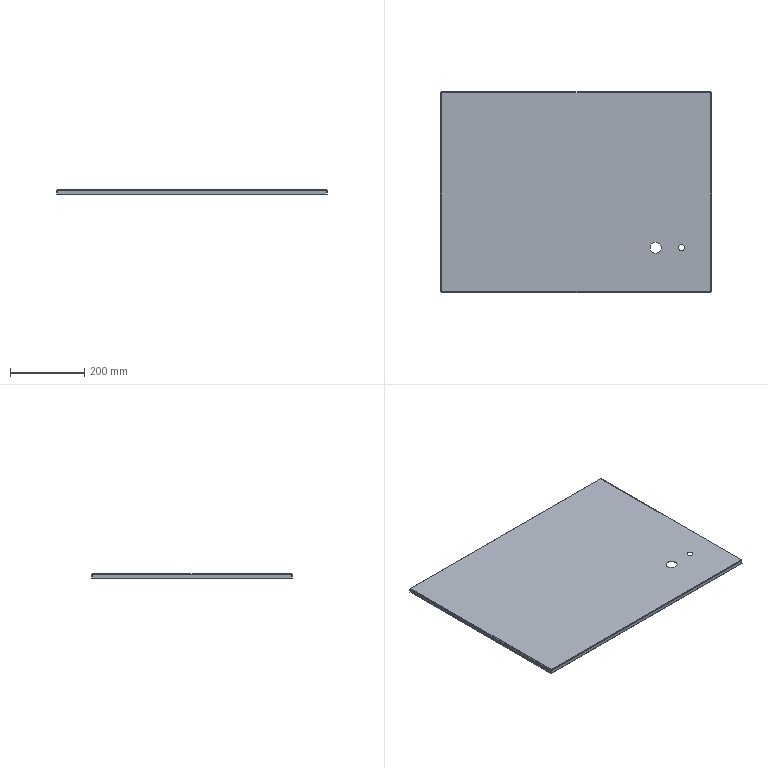Part | SolidWorks | features EdgeFlange 3, FlatPattern 1, ICE 1, SMBaseFlange 1, SMMiteredFlange 1, SheetMetal 1 | 1 solid | 46 faces | box 729.5 x 540 x 11.5 mm | volume 624958 mm3 | plane 34 | cylinder 12 | commonest cylinder face diameters 1.473 x4 4.473 x4 16 x2 30 x2
STEP:
#1=CARTESIAN_POINT('',(276.,-150.,-1.5));
#2=VERTEX_POINT('',#1);
#3=CARTESIAN_POINT('',(292.,-150.,-1.5));
#4=VERTEX_POINT('',#3);
#5=CARTESIAN_POINT('',(284.,-150.,-1.5));
#6=DIRECTION('',(0.,0.,1.));
#7=DIRECTION('',(1.,0.,0.));
#8=AXIS2_PLACEMENT_3D('',#5,#6,#7);
#9=CIRCLE('',#8,8.);
#10=EDGE_CURVE('',#2,#4,#9,.T.);
#11=ORIENTED_EDGE('',*,*,#10,.F.);
#12=CARTESIAN_POINT('',(276.,-150.,0.));
#13=VERTEX_POINT('',#12);
#14=CARTESIAN_POINT('',(276.,-150.,-11.5));
#15=DIRECTION('',(0.,0.,1.));
#16=VECTOR('',#15,1000.);
#17=LINE('',#14,#16);
#18=EDGE_CURVE('',#2,#13,#17,.T.);
#19=ORIENTED_EDGE('',*,*,#18,.T.);
#20=CARTESIAN_POINT('',(292.,-150.,0.));
#21=VERTEX_POINT('',#20);
#22=CARTESIAN_POINT('',(284.,-150.,0.));
#23=DIRECTION('',(0.,0.,1.));
#24=DIRECTION('',(1.,0.,0.));
#25=AXIS2_PLACEMENT_3D('',#22,#23,#24);
#26=CIRCLE('',#25,8.);
#27=EDGE_CURVE('',#13,#21,#26,.T.);
#28=ORIENTED_EDGE('',*,*,#27,.T.);
#29=CARTESIAN_POINT('',(292.,-150.,-11.5));
#30=DIRECTION('',(0.,0.,1.));
#31=VECTOR('',#30,1000.);
#32=LINE('',#29,#31);
#33=EDGE_CURVE('',#4,#21,#32,.T.);
#34=ORIENTED_EDGE('',*,*,#33,.F.);
#35=EDGE_LOOP('',(#11,#19,#28,#34));
#36=FACE_OUTER_BOUND('',#35,.T.);
#37=CARTESIAN_POINT('',(284.,-150.,-11.5));
#38=DIRECTION('',(0.,0.,1.));
#39=DIRECTION('',(1.,0.,0.));
#40=AXIS2_PLACEMENT_3D('',#37,#38,#39);
#41=CYLINDRICAL_SURFACE('',#40,8.);
#42=ADVANCED_FACE('',(#36),#41,.F.);
#43=CARTESIAN_POINT('',(199.,-150.,-1.5));
#44=VERTEX_POINT('',#43);
#45=CARTESIAN_POINT('',(229.,-150.,-1.5));
#46=VERTEX_POINT('',#45);
#47=CARTESIAN_POINT('',(214.,-150.,-1.5));
#48=DIRECTION('',(0.,0.,1.));
#49=DIRECTION('',(1.,0.,0.));
#50=AXIS2_PLACEMENT_3D('',#47,#48,#49);
#51=CIRCLE('',#50,15.);
#52=EDGE_CURVE('',#44,#46,#51,.T.);
#53=ORIENTED_EDGE('',*,*,#52,.F.);
#54=CARTESIAN_POINT('',(199.,-150.,0.));
#55=VERTEX_POINT('',#54);
#56=CARTESIAN_POINT('',(199.,-150.,-11.5));
#57=DIRECTION('',(0.,0.,1.));
#58=VECTOR('',#57,1000.);
#59=LINE('',#56,#58);
#60=EDGE_CURVE('',#44,#55,#59,.T.);
#61=ORIENTED_EDGE('',*,*,#60,.T.);
#62=CARTESIAN_POINT('',(229.,-150.,0.));
#63=VERTEX_POINT('',#62);
#64=CARTESIAN_POINT('',(214.,-150.,0.));
#65=DIRECTION('',(0.,0.,1.));
#66=DIRECTION('',(1.,0.,0.));
#67=AXIS2_PLACEMENT_3D('',#64,#65,#66);
#68=CIRCLE('',#67,15.);
#69=EDGE_CURVE('',#55,#63,#68,.T.);
#70=ORIENTED_EDGE('',*,*,#69,.T.);
#71=CARTESIAN_POINT('',(229.,-150.,-11.5));
#72=DIRECTION('',(0.,0.,1.));
#73=VECTOR('',#72,1000.);
#74=LINE('',#71,#73);
#75=EDGE_CURVE('',#46,#63,#74,.T.);
#76=ORIENTED_EDGE('',*,*,#75,.F.);
#77=EDGE_LOOP('',(#53,#61,#70,#76));
#78=FACE_OUTER_BOUND('',#77,.T.);
#79=CARTESIAN_POINT('',(214.,-150.,-11.5));
#80=DIRECTION('',(0.,0.,1.));
#81=DIRECTION('',(1.,0.,0.));
#82=AXIS2_PLACEMENT_3D('',#79,#80,#81);
#83=CYLINDRICAL_SURFACE('',#82,15.);
#84=ADVANCED_FACE('',(#78),#83,.F.);
#85=CARTESIAN_POINT('',(361.763,268.5,0.));
#86=VERTEX_POINT('',#85);
#87=CARTESIAN_POINT('',(361.763,268.5,-0.1248));
#88=VERTEX_POINT('',#87);
#89=CARTESIAN_POINT('',(361.763,268.5,0.));
#90=DIRECTION('',(0.,0.,-1.));
#91=VECTOR('',#90,1000.);
#92=LINE('',#89,#91);
#93=EDGE_CURVE('',#86,#88,#92,.T.);
#94=ORIENTED_EDGE('',*,*,#93,.T.);
#95=CARTESIAN_POINT('',(361.763,267.763,0.));
#96=VERTEX_POINT('',#95);
#97=CARTESIAN_POINT('',(361.763,267.763,-2.237));
#98=DIRECTION('',(1.,0.,0.));
#99=DIRECTION('',(0.,0.,-1.));
#100=AXIS2_PLACEMENT_3D('',#97,#98,#99);
#101=CIRCLE('',#100,2.237);
#102=EDGE_CURVE('',#88,#96,#101,.T.);
#103=ORIENTED_EDGE('',*,*,#102,.T.);
#104=CARTESIAN_POINT('',(361.763,-2953.5,0.));
#105=DIRECTION('',(0.,1.,0.));
#106=VECTOR('',#105,1000.);
#107=LINE('',#104,#106);
#108=EDGE_CURVE('',#96,#86,#107,.T.);
#109=ORIENTED_EDGE('',*,*,#108,.T.);
#110=EDGE_LOOP('',(#94,#103,#109));
#111=FACE_OUTER_BOUND('',#110,.T.);
#112=CARTESIAN_POINT('',(361.763,268.5,-1.5));
#113=DIRECTION('',(-1.,0.,0.));
#114=DIRECTION('',(0.,0.,1.));
#115=AXIS2_PLACEMENT_3D('',#112,#113,#114);
#116=PLANE('',#115);
#117=ADVANCED_FACE('',(#111),#116,.T.);
#118=CARTESIAN_POINT('',(-363.263,268.5,0.));
#119=VERTEX_POINT('',#118);
#120=CARTESIAN_POINT('',(-363.263,267.763,0.));
#121=VERTEX_POINT('',#120);
#122=CARTESIAN_POINT('',(-363.263,268.5,0.));
#123=DIRECTION('',(0.,-1.,0.));
#124=VECTOR('',#123,1000.);
#125=LINE('',#122,#124);
#126=EDGE_CURVE('',#119,#121,#125,.T.);
#127=ORIENTED_EDGE('',*,*,#126,.T.);
#128=CARTESIAN_POINT('',(-363.263,268.5,-0.1248));
#129=VERTEX_POINT('',#128);
#130=CARTESIAN_POINT('',(-363.263,267.763,-2.237));
#131=DIRECTION('',(-1.,0.,0.));
#132=DIRECTION('',(0.,0.,-1.));
#133=AXIS2_PLACEMENT_3D('',#130,#131,#132);
#134=CIRCLE('',#133,2.237);
#135=EDGE_CURVE('',#121,#129,#134,.T.);
#136=ORIENTED_EDGE('',*,*,#135,.T.);
#137=CARTESIAN_POINT('',(-363.263,268.5,-1.5));
#138=DIRECTION('',(0.,0.,1.));
#139=VECTOR('',#138,1000.);
#140=LINE('',#137,#139);
#141=EDGE_CURVE('',#129,#119,#140,.T.);
#142=ORIENTED_EDGE('',*,*,#141,.T.);
#143=EDGE_LOOP('',(#127,#136,#142));
#144=FACE_OUTER_BOUND('',#143,.T.);
#145=CARTESIAN_POINT('',(-363.263,267.763,-1.5));
#146=DIRECTION('',(1.,0.,0.));
#147=DIRECTION('',(0.,1.,0.));
#148=AXIS2_PLACEMENT_3D('',#145,#146,#147);
#149=PLANE('',#148);
#150=ADVANCED_FACE('',(#144),#149,.T.);
#151=CARTESIAN_POINT('',(284.,-150.,-1.5));
#152=DIRECTION('',(0.,0.,1.));
#153=DIRECTION('',(1.,0.,0.));
#154=AXIS2_PLACEMENT_3D('',#151,#152,#153);
#155=CIRCLE('',#154,8.);
#156=EDGE_CURVE('',#4,#2,#155,.T.);
#157=ORIENTED_EDGE('',*,*,#156,.T.);
#158=ORIENTED_EDGE('',*,*,#10,.T.);
#159=EDGE_LOOP('',(#157,#158));
#160=FACE_BOUND('',#159,.T.);
#161=CARTESIAN_POINT('',(214.,-150.,-1.5));
#162=DIRECTION('',(0.,0.,1.));
#163=DIRECTION('',(1.,0.,0.));
#164=AXIS2_PLACEMENT_3D('',#161,#162,#163);
#165=CIRCLE('',#164,15.);
#166=EDGE_CURVE('',#46,#44,#165,.T.);
#167=ORIENTED_EDGE('',*,*,#166,.T.);
#168=ORIENTED_EDGE('',*,*,#52,.T.);
#169=EDGE_LOOP('',(#167,#168));
#170=FACE_BOUND('',#169,.T.);
#171=CARTESIAN_POINT('',(361.763,267.763,-1.5));
#172=VERTEX_POINT('',#171);
#173=CARTESIAN_POINT('',(-363.263,267.763,-1.5));
#174=VERTEX_POINT('',#173);
#175=CARTESIAN_POINT('',(361.763,267.763,-1.5));
#176=DIRECTION('',(-1.,0.,0.));
#177=VECTOR('',#176,1000.);
#178=LINE('',#175,#177);
#179=EDGE_CURVE('',#172,#174,#178,.T.);
#180=ORIENTED_EDGE('',*,*,#179,.F.);
#181=CARTESIAN_POINT('',(361.763,-267.763,-1.5));
#182=VERTEX_POINT('',#181);
#183=CARTESIAN_POINT('',(361.763,-2953.5,-1.5));
#184=DIRECTION('',(0.,1.,0.));
#185=VECTOR('',#184,1000.);
#186=LINE('',#183,#185);
#187=EDGE_CURVE('',#182,#172,#186,.T.);
#188=ORIENTED_EDGE('',*,*,#187,.F.);
#189=CARTESIAN_POINT('',(-363.263,-267.763,-1.5));
#190=VERTEX_POINT('',#189);
#191=CARTESIAN_POINT('',(-364.,-267.763,-1.5));
#192=DIRECTION('',(1.,0.,0.));
#193=VECTOR('',#192,1000.);
#194=LINE('',#191,#193);
#195=EDGE_CURVE('',#190,#182,#194,.T.);
#196=ORIENTED_EDGE('',*,*,#195,.F.);
#197=CARTESIAN_POINT('',(-363.263,268.5,-1.5));
#198=DIRECTION('',(0.,-1.,0.));
#199=VECTOR('',#198,1000.);
#200=LINE('',#197,#199);
#201=EDGE_CURVE('',#174,#190,#200,.T.);
#202=ORIENTED_EDGE('',*,*,#201,.F.);
#203=EDGE_LOOP('',(#180,#188,#196,#202));
#204=FACE_OUTER_BOUND('',#203,.T.);
#205=CARTESIAN_POINT('',(0.,0.,-1.5));
#206=DIRECTION('',(0.,0.,1.));
#207=DIRECTION('',(1.,0.,0.));
#208=AXIS2_PLACEMENT_3D('',#205,#206,#207);
#209=PLANE('',#208);
#210=ADVANCED_FACE('',(#160,#170,#204),#209,.F.);
#211=CARTESIAN_POINT('',(284.,-150.,0.));
#212=DIRECTION('',(0.,0.,1.));
#213=DIRECTION('',(1.,0.,0.));
#214=AXIS2_PLACEMENT_3D('',#211,#212,#213);
#215=CIRCLE('',#214,8.);
#216=EDGE_CURVE('',#21,#13,#215,.T.);
#217=ORIENTED_EDGE('',*,*,#216,.F.);
#218=ORIENTED_EDGE('',*,*,#27,.F.);
#219=EDGE_LOOP('',(#217,#218));
#220=FACE_BOUND('',#219,.T.);
#221=CARTESIAN_POINT('',(214.,-150.,0.));
#222=DIRECTION('',(0.,0.,1.));
#223=DIRECTION('',(1.,0.,0.));
#224=AXIS2_PLACEMENT_3D('',#221,#222,#223);
#225=CIRCLE('',#224,15.);
#226=EDGE_CURVE('',#63,#55,#225,.T.);
#227=ORIENTED_EDGE('',*,*,#226,.F.);
#228=ORIENTED_EDGE('',*,*,#69,.F.);
#229=EDGE_LOOP('',(#227,#228));
#230=FACE_BOUND('',#229,.T.);
#231=CARTESIAN_POINT('',(361.763,-267.763,0.));
#232=VERTEX_POINT('',#231);
#233=CARTESIAN_POINT('',(361.763,-2953.5,0.));
#234=DIRECTION('',(0.,1.,0.));
#235=VECTOR('',#234,1000.);
#236=LINE('',#233,#235);
#237=EDGE_CURVE('',#232,#96,#236,.T.);
#238=ORIENTED_EDGE('',*,*,#237,.T.);
#239=CARTESIAN_POINT('',(361.763,267.763,0.));
#240=DIRECTION('',(-1.,0.,0.));
#241=VECTOR('',#240,1000.);
#242=LINE('',#239,#241);
#243=EDGE_CURVE('',#96,#121,#242,.T.);
#244=ORIENTED_EDGE('',*,*,#243,.T.);
#245=CARTESIAN_POINT('',(-363.263,-267.763,0.));
#246=VERTEX_POINT('',#245);
#247=CARTESIAN_POINT('',(-363.263,268.5,0.));
#248=DIRECTION('',(0.,-1.,0.));
#249=VECTOR('',#248,1000.);
#250=LINE('',#247,#249);
#251=EDGE_CURVE('',#121,#246,#250,.T.);
#252=ORIENTED_EDGE('',*,*,#251,.T.);
#253=CARTESIAN_POINT('',(-364.,-267.763,0.));
#254=DIRECTION('',(1.,0.,0.));
#255=VECTOR('',#254,1000.);
#256=LINE('',#253,#255);
#257=EDGE_CURVE('',#246,#232,#256,.T.);
#258=ORIENTED_EDGE('',*,*,#257,.T.);
#259=EDGE_LOOP('',(#238,#244,#252,#258));
#260=FACE_OUTER_BOUND('',#259,.T.);
#261=CARTESIAN_POINT('',(0.,0.,0.));
#262=DIRECTION('',(0.,0.,1.));
#263=DIRECTION('',(1.,0.,0.));
#264=AXIS2_PLACEMENT_3D('',#261,#262,#263);
#265=PLANE('',#264);
#266=ADVANCED_FACE('',(#220,#230,#260),#265,.T.);
#267=CARTESIAN_POINT('',(-364.,-267.763,0.));
#268=VERTEX_POINT('',#267);
#269=CARTESIAN_POINT('',(-364.,-267.763,0.));
#270=DIRECTION('',(1.,0.,0.));
#271=VECTOR('',#270,1000.);
#272=LINE('',#269,#271);
#273=EDGE_CURVE('',#268,#246,#272,.T.);
#274=ORIENTED_EDGE('',*,*,#273,.T.);
#275=CARTESIAN_POINT('',(-364.,-267.763,-0.1248));
#276=VERTEX_POINT('',#275);
#277=CARTESIAN_POINT('',(-363.263,-267.763,-2.237));
#278=DIRECTION('',(0.,-1.,0.));
#279=DIRECTION('',(0.,0.,1.));
#280=AXIS2_PLACEMENT_3D('',#277,#278,#279);
#281=CIRCLE('',#280,2.237);
#282=EDGE_CURVE('',#246,#276,#281,.T.);
#283=ORIENTED_EDGE('',*,*,#282,.T.);
#284=CARTESIAN_POINT('',(-364.,-267.763,-1.5));
#285=DIRECTION('',(0.,0.,1.));
#286=VECTOR('',#285,1000.);
#287=LINE('',#284,#286);
#288=EDGE_CURVE('',#276,#268,#287,.T.);
#289=ORIENTED_EDGE('',*,*,#288,.T.);
#290=EDGE_LOOP('',(#274,#283,#289));
#291=FACE_OUTER_BOUND('',#290,.T.);
#292=CARTESIAN_POINT('',(-363.263,-267.763,-1.5));
#293=DIRECTION('',(0.,1.,0.));
#294=DIRECTION('',(-1.,0.,0.));
#295=AXIS2_PLACEMENT_3D('',#292,#293,#294);
#296=PLANE('',#295);
#297=ADVANCED_FACE('',(#291),#296,.T.);
#298=CARTESIAN_POINT('',(361.763,-268.5,0.));
#299=VERTEX_POINT('',#298);
#300=CARTESIAN_POINT('',(361.763,-2953.5,0.));
#301=DIRECTION('',(0.,1.,0.));
#302=VECTOR('',#301,1000.);
#303=LINE('',#300,#302);
#304=EDGE_CURVE('',#299,#232,#303,.T.);
#305=ORIENTED_EDGE('',*,*,#304,.T.);
#306=CARTESIAN_POINT('',(361.763,-268.5,-0.1248));
#307=VERTEX_POINT('',#306);
#308=CARTESIAN_POINT('',(361.763,-267.763,-2.237));
#309=DIRECTION('',(1.,0.,0.));
#310=DIRECTION('',(0.,0.,1.));
#311=AXIS2_PLACEMENT_3D('',#308,#309,#310);
#312=CIRCLE('',#311,2.237);
#313=EDGE_CURVE('',#232,#307,#312,.T.);
#314=ORIENTED_EDGE('',*,*,#313,.T.);
#315=CARTESIAN_POINT('',(361.763,-268.5,0.));
#316=DIRECTION('',(0.,0.,-1.));
#317=VECTOR('',#316,1000.);
#318=LINE('',#315,#317);
#319=EDGE_CURVE('',#299,#307,#318,.T.);
#320=ORIENTED_EDGE('',*,*,#319,.F.);
#321=EDGE_LOOP('',(#305,#314,#320));
#322=FACE_OUTER_BOUND('',#321,.T.);
#323=CARTESIAN_POINT('',(361.763,-267.763,-1.5));
#324=DIRECTION('',(-1.,0.,0.));
#325=DIRECTION('',(0.,-1.,0.));
#326=AXIS2_PLACEMENT_3D('',#323,#324,#325);
#327=PLANE('',#326);
#328=ADVANCED_FACE('',(#322),#327,.T.);
#329=CARTESIAN_POINT('',(364.,268.5,-11.5));
#330=VERTEX_POINT('',#329);
#331=CARTESIAN_POINT('',(362.5,268.5,-11.5));
#332=VERTEX_POINT('',#331);
#333=CARTESIAN_POINT('',(364.,268.5,-11.5));
#334=DIRECTION('',(-1.,0.,0.));
#335=VECTOR('',#334,1000.);
#336=LINE('',#333,#335);
#337=EDGE_CURVE('',#330,#332,#336,.T.);
#338=ORIENTED_EDGE('',*,*,#337,.F.);
#339=CARTESIAN_POINT('',(364.,-268.5,-11.5));
#340=VERTEX_POINT('',#339);
#341=CARTESIAN_POINT('',(364.,-268.5,-11.5));
#342=DIRECTION('',(0.,1.,0.));
#343=VECTOR('',#342,1000.);
#344=LINE('',#341,#343);
#345=EDGE_CURVE('',#340,#330,#344,.T.);
#346=ORIENTED_EDGE('',*,*,#345,.F.);
#347=CARTESIAN_POINT('',(362.5,-268.5,-11.5));
#348=VERTEX_POINT('',#347);
#349=CARTESIAN_POINT('',(364.,-268.5,-11.5));
#350=DIRECTION('',(-1.,0.,0.));
#351=VECTOR('',#350,1000.);
#352=LINE('',#349,#351);
#353=EDGE_CURVE('',#340,#348,#352,.T.);
#354=ORIENTED_EDGE('',*,*,#353,.T.);
#355=CARTESIAN_POINT('',(362.5,-268.5,-11.5));
#356=DIRECTION('',(0.,1.,0.));
#357=VECTOR('',#356,1000.);
#358=LINE('',#355,#357);
#359=EDGE_CURVE('',#348,#332,#358,.T.);
#360=ORIENTED_EDGE('',*,*,#359,.T.);
#361=EDGE_LOOP('',(#338,#346,#354,#360));
#362=FACE_OUTER_BOUND('',#361,.T.);
#363=CARTESIAN_POINT('',(364.,-268.5,-11.5));
#364=DIRECTION('',(0.,0.,1.));
#365=DIRECTION('',(0.,1.,0.));
#366=AXIS2_PLACEMENT_3D('',#363,#364,#365);
#367=PLANE('',#366);
#368=ADVANCED_FACE('',(#362),#367,.F.);
#369=ORIENTED_EDGE('',*,*,#353,.F.);
#370=CARTESIAN_POINT('',(364.,-268.5,-2.237));
#371=VERTEX_POINT('',#370);
#372=CARTESIAN_POINT('',(364.,-268.5,-11.5));
#373=DIRECTION('',(0.,0.,1.));
#374=VECTOR('',#373,1000.);
#375=LINE('',#372,#374);
#376=EDGE_CURVE('',#340,#371,#375,.T.);
#377=ORIENTED_EDGE('',*,*,#376,.T.);
#378=CARTESIAN_POINT('',(362.5,-268.5,-2.237));
#379=VERTEX_POINT('',#378);
#380=CARTESIAN_POINT('',(364.,-268.5,-2.237));
#381=DIRECTION('',(-1.,0.,0.));
#382=VECTOR('',#381,1000.);
#383=LINE('',#380,#382);
#384=EDGE_CURVE('',#371,#379,#383,.T.);
#385=ORIENTED_EDGE('',*,*,#384,.T.);
#386=CARTESIAN_POINT('',(362.5,-268.5,-11.5));
#387=DIRECTION('',(0.,0.,1.));
#388=VECTOR('',#387,1000.);
#389=LINE('',#386,#388);
#390=EDGE_CURVE('',#348,#379,#389,.T.);
#391=ORIENTED_EDGE('',*,*,#390,.F.);
#392=EDGE_LOOP('',(#369,#377,#385,#391));
#393=FACE_OUTER_BOUND('',#392,.T.);
#394=CARTESIAN_POINT('',(364.,-268.5,-11.5));
#395=DIRECTION('',(0.,-1.,0.));
#396=DIRECTION('',(0.,0.,1.));
#397=AXIS2_PLACEMENT_3D('',#394,#395,#396);
#398=PLANE('',#397);
#399=ADVANCED_FACE('',(#393),#398,.T.);
#400=CARTESIAN_POINT('',(364.,268.5,-2.237));
#401=VERTEX_POINT('',#400);
#402=CARTESIAN_POINT('',(364.,268.5,-11.5));
#403=DIRECTION('',(0.,0.,-1.));
#404=VECTOR('',#403,1000.);
#405=LINE('',#402,#404);
#406=EDGE_CURVE('',#401,#330,#405,.T.);
#407=ORIENTED_EDGE('',*,*,#406,.T.);
#408=ORIENTED_EDGE('',*,*,#337,.T.);
#409=CARTESIAN_POINT('',(362.5,268.5,-2.237));
#410=VERTEX_POINT('',#409);
#411=CARTESIAN_POINT('',(362.5,268.5,-11.5));
#412=DIRECTION('',(0.,0.,-1.));
#413=VECTOR('',#412,1000.);
#414=LINE('',#411,#413);
#415=EDGE_CURVE('',#410,#332,#414,.T.);
#416=ORIENTED_EDGE('',*,*,#415,.F.);
#417=CARTESIAN_POINT('',(364.,268.5,-2.237));
#418=DIRECTION('',(-1.,0.,0.));
#419=VECTOR('',#418,1000.);
#420=LINE('',#417,#419);
#421=EDGE_CURVE('',#401,#410,#420,.T.);
#422=ORIENTED_EDGE('',*,*,#421,.F.);
#423=EDGE_LOOP('',(#407,#408,#416,#422));
#424=FACE_OUTER_BOUND('',#423,.T.);
#425=CARTESIAN_POINT('',(364.,268.5,-11.5));
#426=DIRECTION('',(0.,1.,0.));
#427=DIRECTION('',(0.,0.,-1.));
#428=AXIS2_PLACEMENT_3D('',#425,#426,#427);
#429=PLANE('',#428);
#430=ADVANCED_FACE('',(#424),#429,.T.);
#431=CARTESIAN_POINT('',(362.5,-268.5,-2.237));
#432=DIRECTION('',(0.,1.,0.));
#433=VECTOR('',#432,1000.);
#434=LINE('',#431,#433);
#435=EDGE_CURVE('',#379,#410,#434,.T.);
#436=ORIENTED_EDGE('',*,*,#435,.T.);
#437=ORIENTED_EDGE('',*,*,#415,.T.);
#438=ORIENTED_EDGE('',*,*,#359,.F.);
#439=ORIENTED_EDGE('',*,*,#390,.T.);
#440=EDGE_LOOP('',(#436,#437,#438,#439));
#441=FACE_OUTER_BOUND('',#440,.T.);
#442=CARTESIAN_POINT('',(362.5,-268.5,-11.5));
#443=DIRECTION('',(-1.,0.,0.));
#444=DIRECTION('',(0.,0.,1.));
#445=AXIS2_PLACEMENT_3D('',#442,#443,#444);
#446=PLANE('',#445);
#447=ADVANCED_FACE('',(#441),#446,.T.);
#448=CARTESIAN_POINT('',(364.,-268.5,-2.237));
#449=DIRECTION('',(0.,1.,0.));
#450=VECTOR('',#449,1000.);
#451=LINE('',#448,#450);
#452=EDGE_CURVE('',#371,#401,#451,.T.);
#453=ORIENTED_EDGE('',*,*,#452,.F.);
#454=ORIENTED_EDGE('',*,*,#376,.F.);
#455=ORIENTED_EDGE('',*,*,#345,.T.);
#456=ORIENTED_EDGE('',*,*,#406,.F.);
#457=EDGE_LOOP('',(#453,#454,#455,#456));
#458=FACE_OUTER_BOUND('',#457,.T.);
#459=CARTESIAN_POINT('',(364.,-268.5,-11.5));
#460=DIRECTION('',(-1.,0.,0.));
#461=DIRECTION('',(0.,0.,1.));
#462=AXIS2_PLACEMENT_3D('',#459,#460,#461);
#463=PLANE('',#462);
#464=ADVANCED_FACE('',(#458),#463,.F.);
#465=ORIENTED_EDGE('',*,*,#384,.F.);
#466=CARTESIAN_POINT('',(361.763,-268.5,-2.237));
#467=DIRECTION('',(0.,-1.,0.));
#468=DIRECTION('',(1.,0.,0.));
#469=AXIS2_PLACEMENT_3D('',#466,#467,#468);
#470=CIRCLE('',#469,2.237);
#471=EDGE_CURVE('',#371,#299,#470,.T.);
#472=ORIENTED_EDGE('',*,*,#471,.T.);
#473=ORIENTED_EDGE('',*,*,#319,.T.);
#474=CARTESIAN_POINT('',(361.763,-268.5,-1.5));
#475=VERTEX_POINT('',#474);
#476=CARTESIAN_POINT('',(361.763,-268.5,0.));
#477=DIRECTION('',(0.,0.,-1.));
#478=VECTOR('',#477,1000.);
#479=LINE('',#476,#478);
#480=EDGE_CURVE('',#307,#475,#479,.T.);
#481=ORIENTED_EDGE('',*,*,#480,.T.);
#482=CARTESIAN_POINT('',(361.763,-268.5,-2.237));
#483=DIRECTION('',(0.,-1.,0.));
#484=DIRECTION('',(-1.,0.,0.));
#485=AXIS2_PLACEMENT_3D('',#482,#483,#484);
#486=CIRCLE('',#485,0.7366);
#487=EDGE_CURVE('',#379,#475,#486,.T.);
#488=ORIENTED_EDGE('',*,*,#487,.F.);
#489=EDGE_LOOP('',(#465,#472,#473,#481,#488));
#490=FACE_OUTER_BOUND('',#489,.T.);
#491=CARTESIAN_POINT('',(361.763,-268.5,-2.237));
#492=DIRECTION('',(0.,1.,0.));
#493=DIRECTION('',(-1.,0.,0.));
#494=AXIS2_PLACEMENT_3D('',#491,#492,#493);
#495=PLANE('',#494);
#496=ADVANCED_FACE('',(#490),#495,.F.);
#497=CARTESIAN_POINT('',(361.763,268.5,-2.237));
#498=DIRECTION('',(0.,1.,0.));
#499=DIRECTION('',(-1.,0.,0.));
#500=AXIS2_PLACEMENT_3D('',#497,#498,#499);
#501=CIRCLE('',#500,2.237);
#502=EDGE_CURVE('',#86,#401,#501,.T.);
#503=ORIENTED_EDGE('',*,*,#502,.T.);
#504=ORIENTED_EDGE('',*,*,#421,.T.);
#505=CARTESIAN_POINT('',(361.763,268.5,-1.5));
#506=VERTEX_POINT('',#505);
#507=CARTESIAN_POINT('',(361.763,268.5,-2.237));
#508=DIRECTION('',(0.,1.,0.));
#509=DIRECTION('',(-1.,0.,0.));
#510=AXIS2_PLACEMENT_3D('',#507,#508,#509);
#511=CIRCLE('',#510,0.7366);
#512=EDGE_CURVE('',#506,#410,#511,.T.);
#513=ORIENTED_EDGE('',*,*,#512,.F.);
#514=CARTESIAN_POINT('',(361.763,268.5,0.));
#515=DIRECTION('',(0.,0.,-1.));
#516=VECTOR('',#515,1000.);
#517=LINE('',#514,#516);
#518=EDGE_CURVE('',#88,#506,#517,.T.);
#519=ORIENTED_EDGE('',*,*,#518,.F.);
#520=ORIENTED_EDGE('',*,*,#93,.F.);
#521=EDGE_LOOP('',(#503,#504,#513,#519,#520));
#522=FACE_OUTER_BOUND('',#521,.T.);
#523=CARTESIAN_POINT('',(361.763,268.5,-2.237));
#524=DIRECTION('',(0.,-1.,0.));
#525=DIRECTION('',(1.,0.,0.));
#526=AXIS2_PLACEMENT_3D('',#523,#524,#525);
#527=PLANE('',#526);
#528=ADVANCED_FACE('',(#522),#527,.F.);
#529=CARTESIAN_POINT('',(361.763,-2953.5,-1.5));
#530=DIRECTION('',(0.,1.,0.));
#531=VECTOR('',#530,1000.);
#532=LINE('',#529,#531);
#533=EDGE_CURVE('',#475,#182,#532,.T.);
#534=ORIENTED_EDGE('',*,*,#533,.T.);
#535=ORIENTED_EDGE('',*,*,#187,.T.);
#536=CARTESIAN_POINT('',(361.763,268.5,-1.5));
#537=DIRECTION('',(0.,-1.,0.));
#538=VECTOR('',#537,1000.);
#539=LINE('',#536,#538);
#540=EDGE_CURVE('',#506,#172,#539,.T.);
#541=ORIENTED_EDGE('',*,*,#540,.F.);
#542=ORIENTED_EDGE('',*,*,#512,.T.);
#543=ORIENTED_EDGE('',*,*,#435,.F.);
#544=ORIENTED_EDGE('',*,*,#487,.T.);
#545=EDGE_LOOP('',(#534,#535,#541,#542,#543,#544));
#546=FACE_OUTER_BOUND('',#545,.T.);
#547=CARTESIAN_POINT('',(361.763,-2953.5,-2.237));
#548=DIRECTION('',(0.,1.,0.));
#549=DIRECTION('',(-1.,0.,0.));
#550=AXIS2_PLACEMENT_3D('',#547,#548,#549);
#551=CYLINDRICAL_SURFACE('',#550,0.7366);
#552=ADVANCED_FACE('',(#546),#551,.F.);
#553=ORIENTED_EDGE('',*,*,#304,.F.);
#554=ORIENTED_EDGE('',*,*,#471,.F.);
#555=ORIENTED_EDGE('',*,*,#452,.T.);
#556=ORIENTED_EDGE('',*,*,#502,.F.);
#557=ORIENTED_EDGE('',*,*,#108,.F.);
#558=ORIENTED_EDGE('',*,*,#237,.F.);
#559=EDGE_LOOP('',(#553,#554,#555,#556,#557,#558));
#560=FACE_OUTER_BOUND('',#559,.T.);
#561=CARTESIAN_POINT('',(361.763,-2953.5,-2.237));
#562=DIRECTION('',(0.,1.,0.));
#563=DIRECTION('',(-1.,0.,0.));
#564=AXIS2_PLACEMENT_3D('',#561,#562,#563);
#565=CYLINDRICAL_SURFACE('',#564,2.237);
#566=ADVANCED_FACE('',(#560),#565,.T.);
#567=ORIENTED_EDGE('',*,*,#480,.F.);
#568=CARTESIAN_POINT('',(361.763,-270.,-2.237));
#569=VERTEX_POINT('',#568);
#570=CARTESIAN_POINT('',(361.763,-267.763,-2.237));
#571=DIRECTION('',(1.,0.,0.));
#572=DIRECTION('',(0.,0.,1.));
#573=AXIS2_PLACEMENT_3D('',#570,#571,#572);
#574=CIRCLE('',#573,2.237);
#575=EDGE_CURVE('',#307,#569,#574,.T.);
#576=ORIENTED_EDGE('',*,*,#575,.T.);
#577=CARTESIAN_POINT('',(361.763,-268.5,-2.237));
#578=VERTEX_POINT('',#577);
#579=CARTESIAN_POINT('',(361.763,-268.5,-2.237));
#580=DIRECTION('',(0.,-1.,0.));
#581=VECTOR('',#580,1000.);
#582=LINE('',#579,#581);
#583=EDGE_CURVE('',#578,#569,#582,.T.);
#584=ORIENTED_EDGE('',*,*,#583,.F.);
#585=CARTESIAN_POINT('',(361.763,-267.763,-2.237));
#586=DIRECTION('',(1.,0.,0.));
#587=DIRECTION('',(0.,0.,1.));
#588=AXIS2_PLACEMENT_3D('',#585,#586,#587);
#589=CIRCLE('',#588,0.7366);
#590=EDGE_CURVE('',#182,#578,#589,.T.);
#591=ORIENTED_EDGE('',*,*,#590,.F.);
#592=ORIENTED_EDGE('',*,*,#533,.F.);
#593=EDGE_LOOP('',(#567,#576,#584,#591,#592));
#594=FACE_OUTER_BOUND('',#593,.T.);
#595=CARTESIAN_POINT('',(361.763,-267.763,-2.237));
#596=DIRECTION('',(1.,0.,0.));
#597=DIRECTION('',(0.,0.,-1.));
#598=AXIS2_PLACEMENT_3D('',#595,#596,#597);
#599=PLANE('',#598);
#600=ADVANCED_FACE('',(#594),#599,.T.);
#601=CARTESIAN_POINT('',(-364.,-268.5,-2.237));
#602=VERTEX_POINT('',#601);
#603=CARTESIAN_POINT('',(-364.,-267.763,-1.5));
#604=VERTEX_POINT('',#603);
#605=CARTESIAN_POINT('',(-364.,-267.763,-2.237));
#606=DIRECTION('',(-1.,0.,0.));
#607=DIRECTION('',(0.,0.,1.));
#608=AXIS2_PLACEMENT_3D('',#605,#606,#607);
#609=CIRCLE('',#608,0.7366);
#610=EDGE_CURVE('',#602,#604,#609,.T.);
#611=ORIENTED_EDGE('',*,*,#610,.F.);
#612=CARTESIAN_POINT('',(-364.,-270.,-2.237));
#613=VERTEX_POINT('',#612);
#614=CARTESIAN_POINT('',(-364.,-268.5,-2.237));
#615=DIRECTION('',(0.,-1.,0.));
#616=VECTOR('',#615,1000.);
#617=LINE('',#614,#616);
#618=EDGE_CURVE('',#602,#613,#617,.T.);
#619=ORIENTED_EDGE('',*,*,#618,.T.);
#620=CARTESIAN_POINT('',(-364.,-267.763,-2.237));
#621=DIRECTION('',(-1.,0.,0.));
#622=DIRECTION('',(0.,0.,1.));
#623=AXIS2_PLACEMENT_3D('',#620,#621,#622);
#624=CIRCLE('',#623,2.237);
#625=EDGE_CURVE('',#613,#268,#624,.T.);
#626=ORIENTED_EDGE('',*,*,#625,.T.);
#627=ORIENTED_EDGE('',*,*,#288,.F.);
#628=CARTESIAN_POINT('',(-364.,-267.763,-1.5));
#629=DIRECTION('',(0.,0.,1.));
#630=VECTOR('',#629,1000.);
#631=LINE('',#628,#630);
#632=EDGE_CURVE('',#604,#276,#631,.T.);
#633=ORIENTED_EDGE('',*,*,#632,.F.);
#634=EDGE_LOOP('',(#611,#619,#626,#627,#633));
#635=FACE_OUTER_BOUND('',#634,.T.);
#636=CARTESIAN_POINT('',(-364.,-267.763,-2.237));
#637=DIRECTION('',(1.,0.,0.));
#638=DIRECTION('',(0.,0.,-1.));
#639=AXIS2_PLACEMENT_3D('',#636,#637,#638);
#640=PLANE('',#639);
#641=ADVANCED_FACE('',(#635),#640,.F.);
#642=ORIENTED_EDGE('',*,*,#273,.F.);
#643=ORIENTED_EDGE('',*,*,#625,.F.);
#644=CARTESIAN_POINT('',(0.,-270.,-2.237));
#645=DIRECTION('',(1.,0.,0.));
#646=VECTOR('',#645,1000.);
#647=LINE('',#644,#646);
#648=EDGE_CURVE('',#613,#569,#647,.T.);
#649=ORIENTED_EDGE('',*,*,#648,.T.);
#650=ORIENTED_EDGE('',*,*,#575,.F.);
#651=ORIENTED_EDGE('',*,*,#313,.F.);
#652=ORIENTED_EDGE('',*,*,#257,.F.);
#653=EDGE_LOOP('',(#642,#643,#649,#650,#651,#652));
#654=FACE_OUTER_BOUND('',#653,.T.);
#655=CARTESIAN_POINT('',(-364.,-267.763,-2.237));
#656=DIRECTION('',(-1.,0.,0.));
#657=DIRECTION('',(0.,-1.,0.));
#658=AXIS2_PLACEMENT_3D('',#655,#656,#657);
#659=CYLINDRICAL_SURFACE('',#658,2.237);
#660=ADVANCED_FACE('',(#654),#659,.T.);
#661=CARTESIAN_POINT('',(-364.,-267.763,-1.5));
#662=DIRECTION('',(1.,0.,0.));
#663=VECTOR('',#662,1000.);
#664=LINE('',#661,#663);
#665=EDGE_CURVE('',#604,#190,#664,.T.);
#666=ORIENTED_EDGE('',*,*,#665,.T.);
#667=ORIENTED_EDGE('',*,*,#195,.T.);
#668=ORIENTED_EDGE('',*,*,#590,.T.);
#669=CARTESIAN_POINT('',(361.763,-268.5,-2.237));
#670=DIRECTION('',(-1.,0.,0.));
#671=VECTOR('',#670,1000.);
#672=LINE('',#669,#671);
#673=EDGE_CURVE('',#578,#602,#672,.T.);
#674=ORIENTED_EDGE('',*,*,#673,.T.);
#675=ORIENTED_EDGE('',*,*,#610,.T.);
#676=EDGE_LOOP('',(#666,#667,#668,#674,#675));
#677=FACE_OUTER_BOUND('',#676,.T.);
#678=CARTESIAN_POINT('',(-364.,-267.763,-2.237));
#679=DIRECTION('',(-1.,0.,0.));
#680=DIRECTION('',(0.,-1.,0.));
#681=AXIS2_PLACEMENT_3D('',#678,#679,#680);
#682=CYLINDRICAL_SURFACE('',#681,0.7366);
#683=ADVANCED_FACE('',(#677),#682,.F.);
#684=ORIENTED_EDGE('',*,*,#618,.F.);
#685=CARTESIAN_POINT('',(-364.,-268.5,-11.5));
#686=VERTEX_POINT('',#685);
#687=CARTESIAN_POINT('',(-364.,-268.5,-11.5));
#688=DIRECTION('',(0.,0.,-1.));
#689=VECTOR('',#688,1000.);
#690=LINE('',#687,#689);
#691=EDGE_CURVE('',#602,#686,#690,.T.);
#692=ORIENTED_EDGE('',*,*,#691,.T.);
#693=CARTESIAN_POINT('',(-364.,-270.,-11.5));
#694=VERTEX_POINT('',#693);
#695=CARTESIAN_POINT('',(-364.,-270.,-11.5));
#696=DIRECTION('',(0.,1.,0.));
#697=VECTOR('',#696,1000.);
#698=LINE('',#695,#697);
#699=EDGE_CURVE('',#694,#686,#698,.T.);
#700=ORIENTED_EDGE('',*,*,#699,.F.);
#701=CARTESIAN_POINT('',(-364.,-270.,-11.5));
#702=DIRECTION('',(0.,0.,-1.));
#703=VECTOR('',#702,1000.);
#704=LINE('',#701,#703);
#705=EDGE_CURVE('',#613,#694,#704,.T.);
#706=ORIENTED_EDGE('',*,*,#705,.F.);
#707=EDGE_LOOP('',(#684,#692,#700,#706));
#708=FACE_OUTER_BOUND('',#707,.T.);
#709=CARTESIAN_POINT('',(-364.,-270.,-11.5));
#710=DIRECTION('',(1.,0.,0.));
#711=DIRECTION('',(0.,0.,-1.));
#712=AXIS2_PLACEMENT_3D('',#709,#710,#711);
#713=PLANE('',#712);
#714=ADVANCED_FACE('',(#708),#713,.F.);
#715=ORIENTED_EDGE('',*,*,#583,.T.);
#716=CARTESIAN_POINT('',(361.763,-270.,-11.5));
#717=VERTEX_POINT('',#716);
#718=CARTESIAN_POINT('',(361.763,-270.,-1.5));
#719=DIRECTION('',(0.,0.,1.));
#720=VECTOR('',#719,1000.);
#721=LINE('',#718,#720);
#722=EDGE_CURVE('',#717,#569,#721,.T.);
#723=ORIENTED_EDGE('',*,*,#722,.F.);
#724=CARTESIAN_POINT('',(361.763,-268.5,-11.5));
#725=VERTEX_POINT('',#724);
#726=CARTESIAN_POINT('',(361.763,-270.,-11.5));
#727=DIRECTION('',(0.,1.,0.));
#728=VECTOR('',#727,1000.);
#729=LINE('',#726,#728);
#730=EDGE_CURVE('',#717,#725,#729,.T.);
#731=ORIENTED_EDGE('',*,*,#730,.T.);
#732=CARTESIAN_POINT('',(361.763,-268.5,-1.5));
#733=DIRECTION('',(0.,0.,1.));
#734=VECTOR('',#733,1000.);
#735=LINE('',#732,#734);
#736=EDGE_CURVE('',#725,#578,#735,.T.);
#737=ORIENTED_EDGE('',*,*,#736,.T.);
#738=EDGE_LOOP('',(#715,#723,#731,#737));
#739=FACE_OUTER_BOUND('',#738,.T.);
#740=CARTESIAN_POINT('',(361.763,-270.,-1.5));
#741=DIRECTION('',(-1.,0.,0.));
#742=DIRECTION('',(0.,0.,1.));
#743=AXIS2_PLACEMENT_3D('',#740,#741,#742);
#744=PLANE('',#743);
#745=ADVANCED_FACE('',(#739),#744,.F.);
#746=ORIENTED_EDGE('',*,*,#648,.F.);
#747=ORIENTED_EDGE('',*,*,#705,.T.);
#748=CARTESIAN_POINT('',(361.763,-270.,-11.5));
#749=DIRECTION('',(1.,0.,0.));
#750=VECTOR('',#749,1000.);
#751=LINE('',#748,#750);
#752=EDGE_CURVE('',#694,#717,#751,.T.);
#753=ORIENTED_EDGE('',*,*,#752,.T.);
#754=ORIENTED_EDGE('',*,*,#722,.T.);
#755=EDGE_LOOP('',(#746,#747,#753,#754));
#756=FACE_OUTER_BOUND('',#755,.T.);
#757=CARTESIAN_POINT('',(0.,-270.,0.));
#758=DIRECTION('',(0.,1.,0.));
#759=DIRECTION('',(0.,0.,1.));
#760=AXIS2_PLACEMENT_3D('',#757,#758,#759);
#761=PLANE('',#760);
#762=ADVANCED_FACE('',(#756),#761,.F.);
#763=ORIENTED_EDGE('',*,*,#691,.F.);
#764=ORIENTED_EDGE('',*,*,#673,.F.);
#765=ORIENTED_EDGE('',*,*,#736,.F.);
#766=CARTESIAN_POINT('',(361.763,-268.5,-11.5));
#767=DIRECTION('',(1.,0.,0.));
#768=VECTOR('',#767,1000.);
#769=LINE('',#766,#768);
#770=EDGE_CURVE('',#686,#725,#769,.T.);
#771=ORIENTED_EDGE('',*,*,#770,.F.);
#772=EDGE_LOOP('',(#763,#764,#765,#771));
#773=FACE_OUTER_BOUND('',#772,.T.);
#774=CARTESIAN_POINT('',(0.,-268.5,0.));
#775=DIRECTION('',(0.,1.,0.));
#776=DIRECTION('',(0.,0.,1.));
#777=AXIS2_PLACEMENT_3D('',#774,#775,#776);
#778=PLANE('',#777);
#779=ADVANCED_FACE('',(#773),#778,.T.);
#780=ORIENTED_EDGE('',*,*,#770,.T.);
#781=ORIENTED_EDGE('',*,*,#730,.F.);
#782=ORIENTED_EDGE('',*,*,#752,.F.);
#783=ORIENTED_EDGE('',*,*,#699,.T.);
#784=EDGE_LOOP('',(#780,#781,#782,#783));
#785=FACE_OUTER_BOUND('',#784,.T.);
#786=CARTESIAN_POINT('',(361.763,-270.,-11.5));
#787=DIRECTION('',(0.,0.,1.));
#788=DIRECTION('',(0.,-1.,0.));
#789=AXIS2_PLACEMENT_3D('',#786,#787,#788);
#790=PLANE('',#789);
#791=ADVANCED_FACE('',(#785),#790,.F.);
#792=ORIENTED_EDGE('',*,*,#665,.F.);
#793=ORIENTED_EDGE('',*,*,#632,.T.);
#794=CARTESIAN_POINT('',(-365.5,-267.763,-2.237));
#795=VERTEX_POINT('',#794);
#796=CARTESIAN_POINT('',(-363.263,-267.763,-2.237));
#797=DIRECTION('',(0.,-1.,0.));
#798=DIRECTION('',(0.,0.,1.));
#799=AXIS2_PLACEMENT_3D('',#796,#797,#798);
#800=CIRCLE('',#799,2.237);
#801=EDGE_CURVE('',#276,#795,#800,.T.);
#802=ORIENTED_EDGE('',*,*,#801,.T.);
#803=CARTESIAN_POINT('',(-364.,-267.763,-2.237));
#804=VERTEX_POINT('',#803);
#805=CARTESIAN_POINT('',(-364.,-267.763,-2.237));
#806=DIRECTION('',(-1.,0.,0.));
#807=VECTOR('',#806,1000.);
#808=LINE('',#805,#807);
#809=EDGE_CURVE('',#804,#795,#808,.T.);
#810=ORIENTED_EDGE('',*,*,#809,.F.);
#811=CARTESIAN_POINT('',(-363.263,-267.763,-2.237));
#812=DIRECTION('',(0.,-1.,0.));
#813=DIRECTION('',(0.,0.,1.));
#814=AXIS2_PLACEMENT_3D('',#811,#812,#813);
#815=CIRCLE('',#814,0.7366);
#816=EDGE_CURVE('',#190,#804,#815,.T.);
#817=ORIENTED_EDGE('',*,*,#816,.F.);
#818=EDGE_LOOP('',(#792,#793,#802,#810,#817));
#819=FACE_OUTER_BOUND('',#818,.T.);
#820=CARTESIAN_POINT('',(-363.263,-267.763,-2.237));
#821=DIRECTION('',(0.,-1.,0.));
#822=DIRECTION('',(0.,0.,-1.));
#823=AXIS2_PLACEMENT_3D('',#820,#821,#822);
#824=PLANE('',#823);
#825=ADVANCED_FACE('',(#819),#824,.T.);
#826=CARTESIAN_POINT('',(-364.,268.5,-2.237));
#827=VERTEX_POINT('',#826);
#828=CARTESIAN_POINT('',(-363.263,268.5,-1.5));
#829=VERTEX_POINT('',#828);
#830=CARTESIAN_POINT('',(-363.263,268.5,-2.237));
#831=DIRECTION('',(0.,1.,0.));
#832=DIRECTION('',(0.,0.,1.));
#833=AXIS2_PLACEMENT_3D('',#830,#831,#832);
#834=CIRCLE('',#833,0.7366);
#835=EDGE_CURVE('',#827,#829,#834,.T.);
#836=ORIENTED_EDGE('',*,*,#835,.F.);
#837=CARTESIAN_POINT('',(-365.5,268.5,-2.237));
#838=VERTEX_POINT('',#837);
#839=CARTESIAN_POINT('',(-364.,268.5,-2.237));
#840=DIRECTION('',(-1.,0.,0.));
#841=VECTOR('',#840,1000.);
#842=LINE('',#839,#841);
#843=EDGE_CURVE('',#827,#838,#842,.T.);
#844=ORIENTED_EDGE('',*,*,#843,.T.);
#845=CARTESIAN_POINT('',(-363.263,268.5,-2.237));
#846=DIRECTION('',(0.,1.,0.));
#847=DIRECTION('',(0.,0.,1.));
#848=AXIS2_PLACEMENT_3D('',#845,#846,#847);
#849=CIRCLE('',#848,2.237);
#850=EDGE_CURVE('',#838,#119,#849,.T.);
#851=ORIENTED_EDGE('',*,*,#850,.T.);
#852=ORIENTED_EDGE('',*,*,#141,.F.);
#853=CARTESIAN_POINT('',(-363.263,268.5,-1.5));
#854=DIRECTION('',(0.,0.,1.));
#855=VECTOR('',#854,1000.);
#856=LINE('',#853,#855);
#857=EDGE_CURVE('',#829,#129,#856,.T.);
#858=ORIENTED_EDGE('',*,*,#857,.F.);
#859=EDGE_LOOP('',(#836,#844,#851,#852,#858));
#860=FACE_OUTER_BOUND('',#859,.T.);
#861=CARTESIAN_POINT('',(-363.263,268.5,-2.237));
#862=DIRECTION('',(0.,-1.,0.));
#863=DIRECTION('',(0.,0.,-1.));
#864=AXIS2_PLACEMENT_3D('',#861,#862,#863);
#865=PLANE('',#864);
#866=ADVANCED_FACE('',(#860),#865,.F.);
#867=ORIENTED_EDGE('',*,*,#126,.F.);
#868=ORIENTED_EDGE('',*,*,#850,.F.);
#869=CARTESIAN_POINT('',(-365.5,0.,-2.237));
#870=DIRECTION('',(0.,-1.,0.));
#871=VECTOR('',#870,1000.);
#872=LINE('',#869,#871);
#873=EDGE_CURVE('',#838,#795,#872,.T.);
#874=ORIENTED_EDGE('',*,*,#873,.T.);
#875=ORIENTED_EDGE('',*,*,#801,.F.);
#876=ORIENTED_EDGE('',*,*,#282,.F.);
#877=ORIENTED_EDGE('',*,*,#251,.F.);
#878=EDGE_LOOP('',(#867,#868,#874,#875,#876,#877));
#879=FACE_OUTER_BOUND('',#878,.T.);
#880=CARTESIAN_POINT('',(-363.263,268.5,-2.237));
#881=DIRECTION('',(0.,1.,0.));
#882=DIRECTION('',(-1.,0.,0.));
#883=AXIS2_PLACEMENT_3D('',#880,#881,#882);
#884=CYLINDRICAL_SURFACE('',#883,2.237);
#885=ADVANCED_FACE('',(#879),#884,.T.);
#886=CARTESIAN_POINT('',(-363.263,268.5,-1.5));
#887=DIRECTION('',(0.,-1.,0.));
#888=VECTOR('',#887,1000.);
#889=LINE('',#886,#888);
#890=EDGE_CURVE('',#829,#174,#889,.T.);
#891=ORIENTED_EDGE('',*,*,#890,.T.);
#892=ORIENTED_EDGE('',*,*,#201,.T.);
#893=ORIENTED_EDGE('',*,*,#816,.T.);
#894=CARTESIAN_POINT('',(-364.,-267.763,-2.237));
#895=DIRECTION('',(0.,1.,0.));
#896=VECTOR('',#895,1000.);
#897=LINE('',#894,#896);
#898=EDGE_CURVE('',#804,#827,#897,.T.);
#899=ORIENTED_EDGE('',*,*,#898,.T.);
#900=ORIENTED_EDGE('',*,*,#835,.T.);
#901=EDGE_LOOP('',(#891,#892,#893,#899,#900));
#902=FACE_OUTER_BOUND('',#901,.T.);
#903=CARTESIAN_POINT('',(-363.263,268.5,-2.237));
#904=DIRECTION('',(0.,1.,0.));
#905=DIRECTION('',(-1.,0.,0.));
#906=AXIS2_PLACEMENT_3D('',#903,#904,#905);
#907=CYLINDRICAL_SURFACE('',#906,0.7366);
#908=ADVANCED_FACE('',(#902),#907,.F.);
#909=ORIENTED_EDGE('',*,*,#843,.F.);
#910=CARTESIAN_POINT('',(-364.,268.5,-11.5));
#911=VERTEX_POINT('',#910);
#912=CARTESIAN_POINT('',(-364.,268.5,-11.5));
#913=DIRECTION('',(0.,0.,-1.));
#914=VECTOR('',#913,1000.);
#915=LINE('',#912,#914);
#916=EDGE_CURVE('',#827,#911,#915,.T.);
#917=ORIENTED_EDGE('',*,*,#916,.T.);
#918=CARTESIAN_POINT('',(-365.5,268.5,-11.5));
#919=VERTEX_POINT('',#918);
#920=CARTESIAN_POINT('',(-365.5,268.5,-11.5));
#921=DIRECTION('',(1.,0.,0.));
#922=VECTOR('',#921,1000.);
#923=LINE('',#920,#922);
#924=EDGE_CURVE('',#919,#911,#923,.T.);
#925=ORIENTED_EDGE('',*,*,#924,.F.);
#926=CARTESIAN_POINT('',(-365.5,268.5,-11.5));
#927=DIRECTION('',(0.,0.,-1.));
#928=VECTOR('',#927,1000.);
#929=LINE('',#926,#928);
#930=EDGE_CURVE('',#838,#919,#929,.T.);
#931=ORIENTED_EDGE('',*,*,#930,.F.);
#932=EDGE_LOOP('',(#909,#917,#925,#931));
#933=FACE_OUTER_BOUND('',#932,.T.);
#934=CARTESIAN_POINT('',(-365.5,268.5,-11.5));
#935=DIRECTION('',(0.,-1.,0.));
#936=DIRECTION('',(0.,0.,-1.));
#937=AXIS2_PLACEMENT_3D('',#934,#935,#936);
#938=PLANE('',#937);
#939=ADVANCED_FACE('',(#933),#938,.F.);
#940=ORIENTED_EDGE('',*,*,#809,.T.);
#941=CARTESIAN_POINT('',(-365.5,-267.763,-11.5));
#942=VERTEX_POINT('',#941);
#943=CARTESIAN_POINT('',(-365.5,-267.763,-1.5));
#944=DIRECTION('',(0.,0.,1.));
#945=VECTOR('',#944,1000.);
#946=LINE('',#943,#945);
#947=EDGE_CURVE('',#942,#795,#946,.T.);
#948=ORIENTED_EDGE('',*,*,#947,.F.);
#949=CARTESIAN_POINT('',(-364.,-267.763,-11.5));
#950=VERTEX_POINT('',#949);
#951=CARTESIAN_POINT('',(-365.5,-267.763,-11.5));
#952=DIRECTION('',(1.,0.,0.));
#953=VECTOR('',#952,1000.);
#954=LINE('',#951,#953);
#955=EDGE_CURVE('',#942,#950,#954,.T.);
#956=ORIENTED_EDGE('',*,*,#955,.T.);
#957=CARTESIAN_POINT('',(-364.,-267.763,-1.5));
#958=DIRECTION('',(0.,0.,1.));
#959=VECTOR('',#958,1000.);
#960=LINE('',#957,#959);
#961=EDGE_CURVE('',#950,#804,#960,.T.);
#962=ORIENTED_EDGE('',*,*,#961,.T.);
#963=EDGE_LOOP('',(#940,#948,#956,#962));
#964=FACE_OUTER_BOUND('',#963,.T.);
#965=CARTESIAN_POINT('',(-365.5,-267.763,-1.5));
#966=DIRECTION('',(0.,1.,0.));
#967=DIRECTION('',(0.,0.,1.));
#968=AXIS2_PLACEMENT_3D('',#965,#966,#967);
#969=PLANE('',#968);
#970=ADVANCED_FACE('',(#964),#969,.F.);
#971=ORIENTED_EDGE('',*,*,#873,.F.);
#972=ORIENTED_EDGE('',*,*,#930,.T.);
#973=CARTESIAN_POINT('',(-365.5,-267.763,-11.5));
#974=DIRECTION('',(0.,-1.,0.));
#975=VECTOR('',#974,1000.);
#976=LINE('',#973,#975);
#977=EDGE_CURVE('',#919,#942,#976,.T.);
#978=ORIENTED_EDGE('',*,*,#977,.T.);
#979=ORIENTED_EDGE('',*,*,#947,.T.);
#980=EDGE_LOOP('',(#971,#972,#978,#979));
#981=FACE_OUTER_BOUND('',#980,.T.);
#982=CARTESIAN_POINT('',(-365.5,0.,0.));
#983=DIRECTION('',(1.,0.,0.));
#984=DIRECTION('',(0.,0.,-1.));
#985=AXIS2_PLACEMENT_3D('',#982,#983,#984);
#986=PLANE('',#985);
#987=ADVANCED_FACE('',(#981),#986,.F.);
#988=ORIENTED_EDGE('',*,*,#916,.F.);
#989=ORIENTED_EDGE('',*,*,#898,.F.);
#990=ORIENTED_EDGE('',*,*,#961,.F.);
#991=CARTESIAN_POINT('',(-364.,-267.763,-11.5));
#992=DIRECTION('',(0.,-1.,0.));
#993=VECTOR('',#992,1000.);
#994=LINE('',#991,#993);
#995=EDGE_CURVE('',#911,#950,#994,.T.);
#996=ORIENTED_EDGE('',*,*,#995,.F.);
#997=EDGE_LOOP('',(#988,#989,#990,#996));
#998=FACE_OUTER_BOUND('',#997,.T.);
#999=CARTESIAN_POINT('',(-364.,0.,0.));
#1000=DIRECTION('',(1.,0.,0.));
#1001=DIRECTION('',(0.,0.,-1.));
#1002=AXIS2_PLACEMENT_3D('',#999,#1000,#1001);
#1003=PLANE('',#1002);
#1004=ADVANCED_FACE('',(#998),#1003,.T.);
#1005=ORIENTED_EDGE('',*,*,#995,.T.);
#1006=ORIENTED_EDGE('',*,*,#955,.F.);
#1007=ORIENTED_EDGE('',*,*,#977,.F.);
#1008=ORIENTED_EDGE('',*,*,#924,.T.);
#1009=EDGE_LOOP('',(#1005,#1006,#1007,#1008));
#1010=FACE_OUTER_BOUND('',#1009,.T.);
#1011=CARTESIAN_POINT('',(-365.5,-267.763,-11.5));
#1012=DIRECTION('',(0.,0.,1.));
#1013=DIRECTION('',(1.,0.,0.));
#1014=AXIS2_PLACEMENT_3D('',#1011,#1012,#1013);
#1015=PLANE('',#1014);
#1016=ADVANCED_FACE('',(#1010),#1015,.F.);
#1017=ORIENTED_EDGE('',*,*,#890,.F.);
#1018=ORIENTED_EDGE('',*,*,#857,.T.);
#1019=CARTESIAN_POINT('',(-363.263,270.,-2.237));
#1020=VERTEX_POINT('',#1019);
#1021=CARTESIAN_POINT('',(-363.263,267.763,-2.237));
#1022=DIRECTION('',(-1.,0.,0.));
#1023=DIRECTION('',(0.,0.,-1.));
#1024=AXIS2_PLACEMENT_3D('',#1021,#1022,#1023);
#1025=CIRCLE('',#1024,2.237);
#1026=EDGE_CURVE('',#129,#1020,#1025,.T.);
#1027=ORIENTED_EDGE('',*,*,#1026,.T.);
#1028=CARTESIAN_POINT('',(-363.263,268.5,-2.237));
#1029=VERTEX_POINT('',#1028);
#1030=CARTESIAN_POINT('',(-363.263,268.5,-2.237));
#1031=DIRECTION('',(0.,1.,0.));
#1032=VECTOR('',#1031,1000.);
#1033=LINE('',#1030,#1032);
#1034=EDGE_CURVE('',#1029,#1020,#1033,.T.);
#1035=ORIENTED_EDGE('',*,*,#1034,.F.);
#1036=CARTESIAN_POINT('',(-363.263,267.763,-2.237));
#1037=DIRECTION('',(-1.,0.,0.));
#1038=DIRECTION('',(0.,0.,-1.));
#1039=AXIS2_PLACEMENT_3D('',#1036,#1037,#1038);
#1040=CIRCLE('',#1039,0.7366);
#1041=EDGE_CURVE('',#174,#1029,#1040,.T.);
#1042=ORIENTED_EDGE('',*,*,#1041,.F.);
#1043=EDGE_LOOP('',(#1017,#1018,#1027,#1035,#1042));
#1044=FACE_OUTER_BOUND('',#1043,.T.);
#1045=CARTESIAN_POINT('',(-363.263,267.763,-2.237));
#1046=DIRECTION('',(-1.,0.,0.));
#1047=DIRECTION('',(0.,0.,1.));
#1048=AXIS2_PLACEMENT_3D('',#1045,#1046,#1047);
#1049=PLANE('',#1048);
#1050=ADVANCED_FACE('',(#1044),#1049,.T.);
#1051=CARTESIAN_POINT('',(361.763,270.,-2.237));
#1052=VERTEX_POINT('',#1051);
#1053=CARTESIAN_POINT('',(361.763,267.763,-2.237));
#1054=DIRECTION('',(1.,0.,0.));
#1055=DIRECTION('',(0.,0.,-1.));
#1056=AXIS2_PLACEMENT_3D('',#1053,#1054,#1055);
#1057=CIRCLE('',#1056,2.237);
#1058=EDGE_CURVE('',#1052,#88,#1057,.T.);
#1059=ORIENTED_EDGE('',*,*,#1058,.T.);
#1060=ORIENTED_EDGE('',*,*,#518,.T.);
#1061=ORIENTED_EDGE('',*,*,#540,.T.);
#1062=CARTESIAN_POINT('',(361.763,268.5,-2.237));
#1063=VERTEX_POINT('',#1062);
#1064=CARTESIAN_POINT('',(361.763,267.763,-2.237));
#1065=DIRECTION('',(1.,0.,0.));
#1066=DIRECTION('',(0.,0.,-1.));
#1067=AXIS2_PLACEMENT_3D('',#1064,#1065,#1066);
#1068=CIRCLE('',#1067,0.7366);
#1069=EDGE_CURVE('',#1063,#172,#1068,.T.);
#1070=ORIENTED_EDGE('',*,*,#1069,.F.);
#1071=CARTESIAN_POINT('',(361.763,268.5,-2.237));
#1072=DIRECTION('',(0.,1.,0.));
#1073=VECTOR('',#1072,1000.);
#1074=LINE('',#1071,#1073);
#1075=EDGE_CURVE('',#1063,#1052,#1074,.T.);
#1076=ORIENTED_EDGE('',*,*,#1075,.T.);
#1077=EDGE_LOOP('',(#1059,#1060,#1061,#1070,#1076));
#1078=FACE_OUTER_BOUND('',#1077,.T.);
#1079=CARTESIAN_POINT('',(361.763,267.763,-2.237));
#1080=DIRECTION('',(-1.,0.,0.));
#1081=DIRECTION('',(0.,0.,1.));
#1082=AXIS2_PLACEMENT_3D('',#1079,#1080,#1081);
#1083=PLANE('',#1082);
#1084=ADVANCED_FACE('',(#1078),#1083,.F.);
#1085=ORIENTED_EDGE('',*,*,#243,.F.);
#1086=ORIENTED_EDGE('',*,*,#102,.F.);
#1087=ORIENTED_EDGE('',*,*,#1058,.F.);
#1088=CARTESIAN_POINT('',(0.,270.,-2.237));
#1089=DIRECTION('',(-1.,0.,0.));
#1090=VECTOR('',#1089,1000.);
#1091=LINE('',#1088,#1090);
#1092=EDGE_CURVE('',#1052,#1020,#1091,.T.);
#1093=ORIENTED_EDGE('',*,*,#1092,.T.);
#1094=ORIENTED_EDGE('',*,*,#1026,.F.);
#1095=ORIENTED_EDGE('',*,*,#135,.F.);
#1096=EDGE_LOOP('',(#1085,#1086,#1087,#1093,#1094,#1095));
#1097=FACE_OUTER_BOUND('',#1096,.T.);
#1098=CARTESIAN_POINT('',(361.763,267.763,-2.237));
#1099=DIRECTION('',(1.,0.,0.));
#1100=DIRECTION('',(0.,1.,0.));
#1101=AXIS2_PLACEMENT_3D('',#1098,#1099,#1100);
#1102=CYLINDRICAL_SURFACE('',#1101,2.237);
#1103=ADVANCED_FACE('',(#1097),#1102,.T.);
#1104=ORIENTED_EDGE('',*,*,#179,.T.);
#1105=ORIENTED_EDGE('',*,*,#1041,.T.);
#1106=CARTESIAN_POINT('',(-363.263,268.5,-2.237));
#1107=DIRECTION('',(1.,0.,0.));
#1108=VECTOR('',#1107,1000.);
#1109=LINE('',#1106,#1108);
#1110=EDGE_CURVE('',#1029,#1063,#1109,.T.);
#1111=ORIENTED_EDGE('',*,*,#1110,.T.);
#1112=ORIENTED_EDGE('',*,*,#1069,.T.);
#1113=EDGE_LOOP('',(#1104,#1105,#1111,#1112));
#1114=FACE_OUTER_BOUND('',#1113,.T.);
#1115=CARTESIAN_POINT('',(361.763,267.763,-2.237));
#1116=DIRECTION('',(1.,0.,0.));
#1117=DIRECTION('',(0.,1.,0.));
#1118=AXIS2_PLACEMENT_3D('',#1115,#1116,#1117);
#1119=CYLINDRICAL_SURFACE('',#1118,0.7366);
#1120=ADVANCED_FACE('',(#1114),#1119,.F.);
#1121=ORIENTED_EDGE('',*,*,#1075,.F.);
#1122=CARTESIAN_POINT('',(361.763,268.5,-11.5));
#1123=VERTEX_POINT('',#1122);
#1124=CARTESIAN_POINT('',(361.763,268.5,-11.5));
#1125=DIRECTION('',(0.,0.,-1.));
#1126=VECTOR('',#1125,1000.);
#1127=LINE('',#1124,#1126);
#1128=EDGE_CURVE('',#1063,#1123,#1127,.T.);
#1129=ORIENTED_EDGE('',*,*,#1128,.T.);
#1130=CARTESIAN_POINT('',(361.763,270.,-11.5));
#1131=VERTEX_POINT('',#1130);
#1132=CARTESIAN_POINT('',(361.763,270.,-11.5));
#1133=DIRECTION('',(0.,-1.,0.));
#1134=VECTOR('',#1133,1000.);
#1135=LINE('',#1132,#1134);
#1136=EDGE_CURVE('',#1131,#1123,#1135,.T.);
#1137=ORIENTED_EDGE('',*,*,#1136,.F.);
#1138=CARTESIAN_POINT('',(361.763,270.,-11.5));
#1139=DIRECTION('',(0.,0.,-1.));
#1140=VECTOR('',#1139,1000.);
#1141=LINE('',#1138,#1140);
#1142=EDGE_CURVE('',#1052,#1131,#1141,.T.);
#1143=ORIENTED_EDGE('',*,*,#1142,.F.);
#1144=EDGE_LOOP('',(#1121,#1129,#1137,#1143));
#1145=FACE_OUTER_BOUND('',#1144,.T.);
#1146=CARTESIAN_POINT('',(361.763,270.,-11.5));
#1147=DIRECTION('',(-1.,0.,0.));
#1148=DIRECTION('',(0.,-1.,0.));
#1149=AXIS2_PLACEMENT_3D('',#1146,#1147,#1148);
#1150=PLANE('',#1149);
#1151=ADVANCED_FACE('',(#1145),#1150,.F.);
#1152=ORIENTED_EDGE('',*,*,#1034,.T.);
#1153=CARTESIAN_POINT('',(-363.263,270.,-11.5));
#1154=VERTEX_POINT('',#1153);
#1155=CARTESIAN_POINT('',(-363.263,270.,-1.5));
#1156=DIRECTION('',(0.,0.,1.));
#1157=VECTOR('',#1156,1000.);
#1158=LINE('',#1155,#1157);
#1159=EDGE_CURVE('',#1154,#1020,#1158,.T.);
#1160=ORIENTED_EDGE('',*,*,#1159,.F.);
#1161=CARTESIAN_POINT('',(-363.263,268.5,-11.5));
#1162=VERTEX_POINT('',#1161);
#1163=CARTESIAN_POINT('',(-363.263,270.,-11.5));
#1164=DIRECTION('',(0.,-1.,0.));
#1165=VECTOR('',#1164,1000.);
#1166=LINE('',#1163,#1165);
#1167=EDGE_CURVE('',#1154,#1162,#1166,.T.);
#1168=ORIENTED_EDGE('',*,*,#1167,.T.);
#1169=CARTESIAN_POINT('',(-363.263,268.5,-1.5));
#1170=DIRECTION('',(0.,0.,1.));
#1171=VECTOR('',#1170,1000.);
#1172=LINE('',#1169,#1171);
#1173=EDGE_CURVE('',#1162,#1029,#1172,.T.);
#1174=ORIENTED_EDGE('',*,*,#1173,.T.);
#1175=EDGE_LOOP('',(#1152,#1160,#1168,#1174));
#1176=FACE_OUTER_BOUND('',#1175,.T.);
#1177=CARTESIAN_POINT('',(-363.263,270.,-1.5));
#1178=DIRECTION('',(1.,0.,0.));
#1179=DIRECTION('',(0.,1.,0.));
#1180=AXIS2_PLACEMENT_3D('',#1177,#1178,#1179);
#1181=PLANE('',#1180);
#1182=ADVANCED_FACE('',(#1176),#1181,.F.);
#1183=ORIENTED_EDGE('',*,*,#1092,.F.);
#1184=ORIENTED_EDGE('',*,*,#1142,.T.);
#1185=CARTESIAN_POINT('',(-363.263,270.,-11.5));
#1186=DIRECTION('',(-1.,0.,0.));
#1187=VECTOR('',#1186,1000.);
#1188=LINE('',#1185,#1187);
#1189=EDGE_CURVE('',#1131,#1154,#1188,.T.);
#1190=ORIENTED_EDGE('',*,*,#1189,.T.);
#1191=ORIENTED_EDGE('',*,*,#1159,.T.);
#1192=EDGE_LOOP('',(#1183,#1184,#1190,#1191));
#1193=FACE_OUTER_BOUND('',#1192,.T.);
#1194=CARTESIAN_POINT('',(0.,270.,0.));
#1195=DIRECTION('',(0.,-1.,0.));
#1196=DIRECTION('',(1.,0.,0.));
#1197=AXIS2_PLACEMENT_3D('',#1194,#1195,#1196);
#1198=PLANE('',#1197);
#1199=ADVANCED_FACE('',(#1193),#1198,.F.);
#1200=ORIENTED_EDGE('',*,*,#1128,.F.);
#1201=ORIENTED_EDGE('',*,*,#1110,.F.);
#1202=ORIENTED_EDGE('',*,*,#1173,.F.);
#1203=CARTESIAN_POINT('',(-363.263,268.5,-11.5));
#1204=DIRECTION('',(-1.,0.,0.));
#1205=VECTOR('',#1204,1000.);
#1206=LINE('',#1203,#1205);
#1207=EDGE_CURVE('',#1123,#1162,#1206,.T.);
#1208=ORIENTED_EDGE('',*,*,#1207,.F.);
#1209=EDGE_LOOP('',(#1200,#1201,#1202,#1208));
#1210=FACE_OUTER_BOUND('',#1209,.T.);
#1211=CARTESIAN_POINT('',(0.,268.5,0.));
#1212=DIRECTION('',(0.,-1.,0.));
#1213=DIRECTION('',(1.,0.,0.));
#1214=AXIS2_PLACEMENT_3D('',#1211,#1212,#1213);
#1215=PLANE('',#1214);
#1216=ADVANCED_FACE('',(#1210),#1215,.T.);
#1217=ORIENTED_EDGE('',*,*,#1207,.T.);
#1218=ORIENTED_EDGE('',*,*,#1167,.F.);
#1219=ORIENTED_EDGE('',*,*,#1189,.F.);
#1220=ORIENTED_EDGE('',*,*,#1136,.T.);
#1221=EDGE_LOOP('',(#1217,#1218,#1219,#1220));
#1222=FACE_OUTER_BOUND('',#1221,.T.);
#1223=CARTESIAN_POINT('',(-363.263,270.,-11.5));
#1224=DIRECTION('',(0.,0.,1.));
#1225=DIRECTION('',(0.,-1.,0.));
#1226=AXIS2_PLACEMENT_3D('',#1223,#1224,#1225);
#1227=PLANE('',#1226);
#1228=ADVANCED_FACE('',(#1222),#1227,.F.);
#1229=ORIENTED_EDGE('',*,*,#60,.F.);
#1230=ORIENTED_EDGE('',*,*,#166,.F.);
#1231=ORIENTED_EDGE('',*,*,#75,.T.);
#1232=ORIENTED_EDGE('',*,*,#226,.T.);
#1233=EDGE_LOOP('',(#1229,#1230,#1231,#1232));
#1234=FACE_OUTER_BOUND('',#1233,.T.);
#1235=CARTESIAN_POINT('',(214.,-150.,-11.5));
#1236=DIRECTION('',(0.,0.,1.));
#1237=DIRECTION('',(1.,0.,0.));
#1238=AXIS2_PLACEMENT_3D('',#1235,#1236,#1237);
#1239=CYLINDRICAL_SURFACE('',#1238,15.);
#1240=ADVANCED_FACE('',(#1234),#1239,.F.);
#1241=ORIENTED_EDGE('',*,*,#18,.F.);
#1242=ORIENTED_EDGE('',*,*,#156,.F.);
#1243=ORIENTED_EDGE('',*,*,#33,.T.);
#1244=ORIENTED_EDGE('',*,*,#216,.T.);
#1245=EDGE_LOOP('',(#1241,#1242,#1243,#1244));
#1246=FACE_OUTER_BOUND('',#1245,.T.);
#1247=CARTESIAN_POINT('',(284.,-150.,-11.5));
#1248=DIRECTION('',(0.,0.,1.));
#1249=DIRECTION('',(1.,0.,0.));
#1250=AXIS2_PLACEMENT_3D('',#1247,#1248,#1249);
#1251=CYLINDRICAL_SURFACE('',#1250,8.);
#1252=ADVANCED_FACE('',(#1246),#1251,.F.);
#1253=CLOSED_SHELL('',(#42,#84,#117,#150,#210,#266,#297,#328,#368,#399,#430,#447,#464,#496,#528,#552,#566,#600,#641,#660,#683,#714,#745,#762,#779,#791,#825,#866,#885,#908,#939,#970,#987,#1004,#1016,#1050,#1084,#1103,#1120,#1151,#1182,#1199,#1216,#1228,#1240,#1252));
#1254=MANIFOLD_SOLID_BREP('',#1253);
#1255=CARTESIAN_POINT('',(0.,0.,0.));
#1256=DIRECTION('',(0.,0.,1.));
#1257=DIRECTION('',(1.,0.,0.));
#1258=AXIS2_PLACEMENT_3D('',#1255,#1256,#1257);
#1259=(LENGTH_UNIT()NAMED_UNIT(*)SI_UNIT(.MILLI.,.METRE.));
#1260=UNCERTAINTY_MEASURE_WITH_UNIT(LENGTH_MEASURE(0.00001),#1259,'','');
#1261=(NAMED_UNIT(*)PLANE_ANGLE_UNIT()SI_UNIT($,.RADIAN.));
#1262=(NAMED_UNIT(*)SI_UNIT($,.STERADIAN.)SOLID_ANGLE_UNIT());
#1263=(GEOMETRIC_REPRESENTATION_CONTEXT(3)GLOBAL_UNCERTAINTY_ASSIGNED_CONTEXT((#1260))GLOBAL_UNIT_ASSIGNED_CONTEXT((#1259,#1261,#1262))REPRESENTATION_CONTEXT('',''));
#1264=ADVANCED_BREP_SHAPE_REPRESENTATION('',(#1254,#1258),#1263);